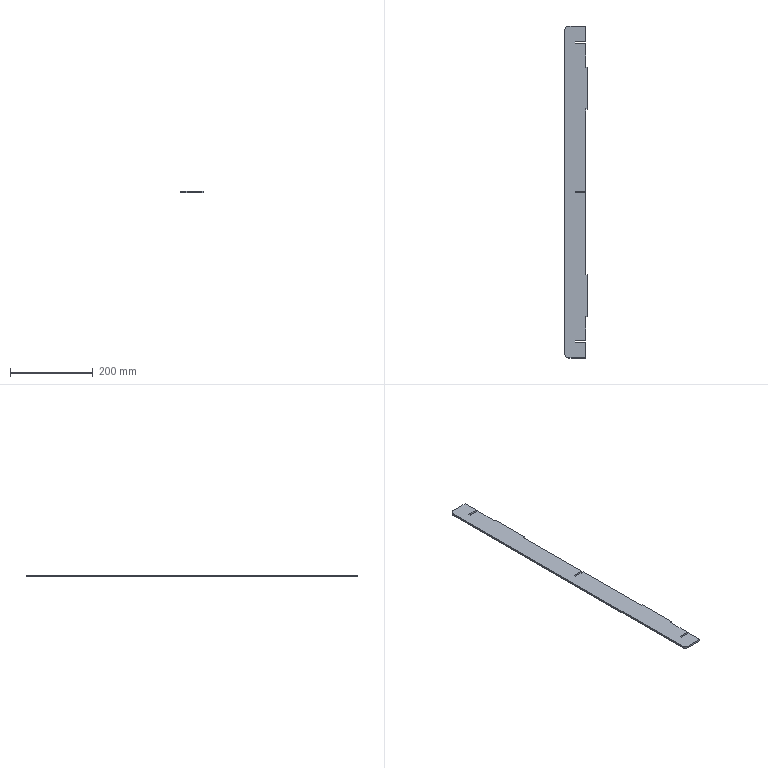Part | SolidWorks | features FlatPattern 1, SMBaseFlange 1, SheetMetal 1 | 1 solid | 28 faces | box 54 x 800 x 4.5 mm | volume 181888 mm3 | plane 26 | cylinder 2 | commonest cylinder face diameters 20 x2
STEP:
#1=CARTESIAN_POINT('',(1108.071,318.842,0.));
#2=VERTEX_POINT('',#1);
#3=CARTESIAN_POINT('',(1108.071,356.592,0.));
#4=VERTEX_POINT('',#3);
#5=CARTESIAN_POINT('',(1108.071,356.592,0.));
#6=DIRECTION('',(0.,1.,0.));
#7=VECTOR('',#6,1000.);
#8=LINE('',#5,#7);
#9=EDGE_CURVE('',#2,#4,#8,.T.);
#10=ORIENTED_EDGE('',*,*,#9,.F.);
#11=CARTESIAN_POINT('',(1108.071,318.842,-4.5));
#12=VERTEX_POINT('',#11);
#13=CARTESIAN_POINT('',(1108.071,318.842,-4.5));
#14=DIRECTION('',(0.,0.,1.));
#15=VECTOR('',#14,1000.);
#16=LINE('',#13,#15);
#17=EDGE_CURVE('',#12,#2,#16,.T.);
#18=ORIENTED_EDGE('',*,*,#17,.F.);
#19=CARTESIAN_POINT('',(1108.071,356.592,-4.5));
#20=VERTEX_POINT('',#19);
#21=CARTESIAN_POINT('',(1108.071,356.592,-4.5));
#22=DIRECTION('',(0.,1.,0.));
#23=VECTOR('',#22,1000.);
#24=LINE('',#21,#23);
#25=EDGE_CURVE('',#12,#20,#24,.T.);
#26=ORIENTED_EDGE('',*,*,#25,.T.);
#27=CARTESIAN_POINT('',(1108.071,356.592,-4.5));
#28=DIRECTION('',(0.,0.,1.));
#29=VECTOR('',#28,1000.);
#30=LINE('',#27,#29);
#31=EDGE_CURVE('',#20,#4,#30,.T.);
#32=ORIENTED_EDGE('',*,*,#31,.T.);
#33=EDGE_LOOP('',(#10,#18,#26,#32));
#34=FACE_OUTER_BOUND('',#33,.T.);
#35=CARTESIAN_POINT('',(1108.071,356.592,-4.5));
#36=DIRECTION('',(1.,0.,0.));
#37=DIRECTION('',(0.,0.,-1.));
#38=AXIS2_PLACEMENT_3D('',#35,#36,#37);
#39=PLANE('',#38);
#40=ADVANCED_FACE('',(#34),#39,.T.);
#41=CARTESIAN_POINT('',(1083.071,318.842,0.));
#42=VERTEX_POINT('',#41);
#43=CARTESIAN_POINT('',(1108.071,318.842,0.));
#44=DIRECTION('',(1.,0.,0.));
#45=VECTOR('',#44,1000.);
#46=LINE('',#43,#45);
#47=EDGE_CURVE('',#42,#2,#46,.T.);
#48=ORIENTED_EDGE('',*,*,#47,.F.);
#49=CARTESIAN_POINT('',(1083.071,318.842,-4.5));
#50=VERTEX_POINT('',#49);
#51=CARTESIAN_POINT('',(1083.071,318.842,-4.5));
#52=DIRECTION('',(0.,0.,1.));
#53=VECTOR('',#52,1000.);
#54=LINE('',#51,#53);
#55=EDGE_CURVE('',#50,#42,#54,.T.);
#56=ORIENTED_EDGE('',*,*,#55,.F.);
#57=CARTESIAN_POINT('',(1108.071,318.842,-4.5));
#58=DIRECTION('',(1.,0.,0.));
#59=VECTOR('',#58,1000.);
#60=LINE('',#57,#59);
#61=EDGE_CURVE('',#50,#12,#60,.T.);
#62=ORIENTED_EDGE('',*,*,#61,.T.);
#63=ORIENTED_EDGE('',*,*,#17,.T.);
#64=EDGE_LOOP('',(#48,#56,#62,#63));
#65=FACE_OUTER_BOUND('',#64,.T.);
#66=CARTESIAN_POINT('',(1108.071,318.842,-4.5));
#67=DIRECTION('',(0.,-1.,0.));
#68=DIRECTION('',(0.,0.,-1.));
#69=AXIS2_PLACEMENT_3D('',#66,#67,#68);
#70=PLANE('',#69);
#71=ADVANCED_FACE('',(#65),#70,.T.);
#72=CARTESIAN_POINT('',(1083.071,314.342,0.));
#73=VERTEX_POINT('',#72);
#74=CARTESIAN_POINT('',(1083.071,318.842,0.));
#75=DIRECTION('',(0.,1.,0.));
#76=VECTOR('',#75,1000.);
#77=LINE('',#74,#76);
#78=EDGE_CURVE('',#73,#42,#77,.T.);
#79=ORIENTED_EDGE('',*,*,#78,.F.);
#80=CARTESIAN_POINT('',(1083.071,314.342,-4.5));
#81=VERTEX_POINT('',#80);
#82=CARTESIAN_POINT('',(1083.071,314.342,-4.5));
#83=DIRECTION('',(0.,0.,1.));
#84=VECTOR('',#83,1000.);
#85=LINE('',#82,#84);
#86=EDGE_CURVE('',#81,#73,#85,.T.);
#87=ORIENTED_EDGE('',*,*,#86,.F.);
#88=CARTESIAN_POINT('',(1083.071,318.842,-4.5));
#89=DIRECTION('',(0.,1.,0.));
#90=VECTOR('',#89,1000.);
#91=LINE('',#88,#90);
#92=EDGE_CURVE('',#81,#50,#91,.T.);
#93=ORIENTED_EDGE('',*,*,#92,.T.);
#94=ORIENTED_EDGE('',*,*,#55,.T.);
#95=EDGE_LOOP('',(#79,#87,#93,#94));
#96=FACE_OUTER_BOUND('',#95,.T.);
#97=CARTESIAN_POINT('',(1083.071,318.842,-4.5));
#98=DIRECTION('',(1.,0.,0.));
#99=DIRECTION('',(0.,0.,-1.));
#100=AXIS2_PLACEMENT_3D('',#97,#98,#99);
#101=PLANE('',#100);
#102=ADVANCED_FACE('',(#96),#101,.T.);
#103=CARTESIAN_POINT('',(1108.071,314.342,0.));
#104=VERTEX_POINT('',#103);
#105=CARTESIAN_POINT('',(1083.071,314.342,0.));
#106=DIRECTION('',(-1.,0.,0.));
#107=VECTOR('',#106,1000.);
#108=LINE('',#105,#107);
#109=EDGE_CURVE('',#104,#73,#108,.T.);
#110=ORIENTED_EDGE('',*,*,#109,.F.);
#111=CARTESIAN_POINT('',(1108.071,314.342,-4.5));
#112=VERTEX_POINT('',#111);
#113=CARTESIAN_POINT('',(1108.071,314.342,-4.5));
#114=DIRECTION('',(0.,0.,1.));
#115=VECTOR('',#114,1000.);
#116=LINE('',#113,#115);
#117=EDGE_CURVE('',#112,#104,#116,.T.);
#118=ORIENTED_EDGE('',*,*,#117,.F.);
#119=CARTESIAN_POINT('',(1083.071,314.342,-4.5));
#120=DIRECTION('',(-1.,0.,0.));
#121=VECTOR('',#120,1000.);
#122=LINE('',#119,#121);
#123=EDGE_CURVE('',#112,#81,#122,.T.);
#124=ORIENTED_EDGE('',*,*,#123,.T.);
#125=ORIENTED_EDGE('',*,*,#86,.T.);
#126=EDGE_LOOP('',(#110,#118,#124,#125));
#127=FACE_OUTER_BOUND('',#126,.T.);
#128=CARTESIAN_POINT('',(1083.071,314.342,-4.5));
#129=DIRECTION('',(0.,1.,0.));
#130=DIRECTION('',(0.,0.,1.));
#131=AXIS2_PLACEMENT_3D('',#128,#129,#130);
#132=PLANE('',#131);
#133=ADVANCED_FACE('',(#127),#132,.T.);
#134=CARTESIAN_POINT('',(1108.071,256.592,0.));
#135=VERTEX_POINT('',#134);
#136=CARTESIAN_POINT('',(1108.071,314.342,0.));
#137=DIRECTION('',(0.,1.,0.));
#138=VECTOR('',#137,1000.);
#139=LINE('',#136,#138);
#140=EDGE_CURVE('',#135,#104,#139,.T.);
#141=ORIENTED_EDGE('',*,*,#140,.F.);
#142=CARTESIAN_POINT('',(1108.071,256.592,-4.5));
#143=VERTEX_POINT('',#142);
#144=CARTESIAN_POINT('',(1108.071,256.592,-4.5));
#145=DIRECTION('',(0.,0.,1.));
#146=VECTOR('',#145,1000.);
#147=LINE('',#144,#146);
#148=EDGE_CURVE('',#143,#135,#147,.T.);
#149=ORIENTED_EDGE('',*,*,#148,.F.);
#150=CARTESIAN_POINT('',(1108.071,314.342,-4.5));
#151=DIRECTION('',(0.,1.,0.));
#152=VECTOR('',#151,1000.);
#153=LINE('',#150,#152);
#154=EDGE_CURVE('',#143,#112,#153,.T.);
#155=ORIENTED_EDGE('',*,*,#154,.T.);
#156=ORIENTED_EDGE('',*,*,#117,.T.);
#157=EDGE_LOOP('',(#141,#149,#155,#156));
#158=FACE_OUTER_BOUND('',#157,.T.);
#159=CARTESIAN_POINT('',(1108.071,314.342,-4.5));
#160=DIRECTION('',(1.,0.,0.));
#161=DIRECTION('',(0.,0.,-1.));
#162=AXIS2_PLACEMENT_3D('',#159,#160,#161);
#163=PLANE('',#162);
#164=ADVANCED_FACE('',(#158),#163,.T.);
#165=CARTESIAN_POINT('',(1112.071,256.592,0.));
#166=VERTEX_POINT('',#165);
#167=CARTESIAN_POINT('',(1108.071,256.592,0.));
#168=DIRECTION('',(-1.,0.,0.));
#169=VECTOR('',#168,1000.);
#170=LINE('',#167,#169);
#171=EDGE_CURVE('',#166,#135,#170,.T.);
#172=ORIENTED_EDGE('',*,*,#171,.F.);
#173=CARTESIAN_POINT('',(1112.071,256.592,-4.5));
#174=VERTEX_POINT('',#173);
#175=CARTESIAN_POINT('',(1112.071,256.592,-4.5));
#176=DIRECTION('',(0.,0.,1.));
#177=VECTOR('',#176,1000.);
#178=LINE('',#175,#177);
#179=EDGE_CURVE('',#174,#166,#178,.T.);
#180=ORIENTED_EDGE('',*,*,#179,.F.);
#181=CARTESIAN_POINT('',(1108.071,256.592,-4.5));
#182=DIRECTION('',(-1.,0.,0.));
#183=VECTOR('',#182,1000.);
#184=LINE('',#181,#183);
#185=EDGE_CURVE('',#174,#143,#184,.T.);
#186=ORIENTED_EDGE('',*,*,#185,.T.);
#187=ORIENTED_EDGE('',*,*,#148,.T.);
#188=EDGE_LOOP('',(#172,#180,#186,#187));
#189=FACE_OUTER_BOUND('',#188,.T.);
#190=CARTESIAN_POINT('',(1108.071,256.592,-4.5));
#191=DIRECTION('',(0.,1.,0.));
#192=DIRECTION('',(0.,0.,1.));
#193=AXIS2_PLACEMENT_3D('',#190,#191,#192);
#194=PLANE('',#193);
#195=ADVANCED_FACE('',(#189),#194,.T.);
#196=CARTESIAN_POINT('',(1112.071,156.592,0.));
#197=VERTEX_POINT('',#196);
#198=CARTESIAN_POINT('',(1112.071,256.592,0.));
#199=DIRECTION('',(0.,1.,0.));
#200=VECTOR('',#199,1000.);
#201=LINE('',#198,#200);
#202=EDGE_CURVE('',#197,#166,#201,.T.);
#203=ORIENTED_EDGE('',*,*,#202,.F.);
#204=CARTESIAN_POINT('',(1112.071,156.592,-4.5));
#205=VERTEX_POINT('',#204);
#206=CARTESIAN_POINT('',(1112.071,156.592,-4.5));
#207=DIRECTION('',(0.,0.,1.));
#208=VECTOR('',#207,1000.);
#209=LINE('',#206,#208);
#210=EDGE_CURVE('',#205,#197,#209,.T.);
#211=ORIENTED_EDGE('',*,*,#210,.F.);
#212=CARTESIAN_POINT('',(1112.071,256.592,-4.5));
#213=DIRECTION('',(0.,1.,0.));
#214=VECTOR('',#213,1000.);
#215=LINE('',#212,#214);
#216=EDGE_CURVE('',#205,#174,#215,.T.);
#217=ORIENTED_EDGE('',*,*,#216,.T.);
#218=ORIENTED_EDGE('',*,*,#179,.T.);
#219=EDGE_LOOP('',(#203,#211,#217,#218));
#220=FACE_OUTER_BOUND('',#219,.T.);
#221=CARTESIAN_POINT('',(1112.071,256.592,-4.5));
#222=DIRECTION('',(1.,0.,0.));
#223=DIRECTION('',(0.,1.,0.));
#224=AXIS2_PLACEMENT_3D('',#221,#222,#223);
#225=PLANE('',#224);
#226=ADVANCED_FACE('',(#220),#225,.T.);
#227=CARTESIAN_POINT('',(1108.071,156.592,0.));
#228=VERTEX_POINT('',#227);
#229=CARTESIAN_POINT('',(1112.071,156.592,0.));
#230=DIRECTION('',(1.,0.,0.));
#231=VECTOR('',#230,1000.);
#232=LINE('',#229,#231);
#233=EDGE_CURVE('',#228,#197,#232,.T.);
#234=ORIENTED_EDGE('',*,*,#233,.F.);
#235=CARTESIAN_POINT('',(1108.071,156.592,-4.5));
#236=VERTEX_POINT('',#235);
#237=CARTESIAN_POINT('',(1108.071,156.592,-4.5));
#238=DIRECTION('',(0.,0.,1.));
#239=VECTOR('',#238,1000.);
#240=LINE('',#237,#239);
#241=EDGE_CURVE('',#236,#228,#240,.T.);
#242=ORIENTED_EDGE('',*,*,#241,.F.);
#243=CARTESIAN_POINT('',(1112.071,156.592,-4.5));
#244=DIRECTION('',(1.,0.,0.));
#245=VECTOR('',#244,1000.);
#246=LINE('',#243,#245);
#247=EDGE_CURVE('',#236,#205,#246,.T.);
#248=ORIENTED_EDGE('',*,*,#247,.T.);
#249=ORIENTED_EDGE('',*,*,#210,.T.);
#250=EDGE_LOOP('',(#234,#242,#248,#249));
#251=FACE_OUTER_BOUND('',#250,.T.);
#252=CARTESIAN_POINT('',(1112.071,156.592,-4.5));
#253=DIRECTION('',(0.,-1.,0.));
#254=DIRECTION('',(0.,0.,-1.));
#255=AXIS2_PLACEMENT_3D('',#252,#253,#254);
#256=PLANE('',#255);
#257=ADVANCED_FACE('',(#251),#256,.T.);
#258=CARTESIAN_POINT('',(1108.071,-41.158,0.));
#259=VERTEX_POINT('',#258);
#260=CARTESIAN_POINT('',(1108.071,156.592,0.));
#261=DIRECTION('',(0.,1.,0.));
#262=VECTOR('',#261,1000.);
#263=LINE('',#260,#262);
#264=EDGE_CURVE('',#259,#228,#263,.T.);
#265=ORIENTED_EDGE('',*,*,#264,.F.);
#266=CARTESIAN_POINT('',(1108.071,-41.158,-4.5));
#267=VERTEX_POINT('',#266);
#268=CARTESIAN_POINT('',(1108.071,-41.158,-4.5));
#269=DIRECTION('',(0.,0.,1.));
#270=VECTOR('',#269,1000.);
#271=LINE('',#268,#270);
#272=EDGE_CURVE('',#267,#259,#271,.T.);
#273=ORIENTED_EDGE('',*,*,#272,.F.);
#274=CARTESIAN_POINT('',(1108.071,156.592,-4.5));
#275=DIRECTION('',(0.,1.,0.));
#276=VECTOR('',#275,1000.);
#277=LINE('',#274,#276);
#278=EDGE_CURVE('',#267,#236,#277,.T.);
#279=ORIENTED_EDGE('',*,*,#278,.T.);
#280=ORIENTED_EDGE('',*,*,#241,.T.);
#281=EDGE_LOOP('',(#265,#273,#279,#280));
#282=FACE_OUTER_BOUND('',#281,.T.);
#283=CARTESIAN_POINT('',(1108.071,156.592,-4.5));
#284=DIRECTION('',(1.,0.,0.));
#285=DIRECTION('',(0.,0.,-1.));
#286=AXIS2_PLACEMENT_3D('',#283,#284,#285);
#287=PLANE('',#286);
#288=ADVANCED_FACE('',(#282),#287,.T.);
#289=CARTESIAN_POINT('',(1083.071,-41.158,0.));
#290=VERTEX_POINT('',#289);
#291=CARTESIAN_POINT('',(1108.071,-41.158,0.));
#292=DIRECTION('',(1.,0.,0.));
#293=VECTOR('',#292,1000.);
#294=LINE('',#291,#293);
#295=EDGE_CURVE('',#290,#259,#294,.T.);
#296=ORIENTED_EDGE('',*,*,#295,.F.);
#297=CARTESIAN_POINT('',(1083.071,-41.158,-4.5));
#298=VERTEX_POINT('',#297);
#299=CARTESIAN_POINT('',(1083.071,-41.158,-4.5));
#300=DIRECTION('',(0.,0.,1.));
#301=VECTOR('',#300,1000.);
#302=LINE('',#299,#301);
#303=EDGE_CURVE('',#298,#290,#302,.T.);
#304=ORIENTED_EDGE('',*,*,#303,.F.);
#305=CARTESIAN_POINT('',(1108.071,-41.158,-4.5));
#306=DIRECTION('',(1.,0.,0.));
#307=VECTOR('',#306,1000.);
#308=LINE('',#305,#307);
#309=EDGE_CURVE('',#298,#267,#308,.T.);
#310=ORIENTED_EDGE('',*,*,#309,.T.);
#311=ORIENTED_EDGE('',*,*,#272,.T.);
#312=EDGE_LOOP('',(#296,#304,#310,#311));
#313=FACE_OUTER_BOUND('',#312,.T.);
#314=CARTESIAN_POINT('',(1108.071,-41.158,-4.5));
#315=DIRECTION('',(0.,-1.,0.));
#316=DIRECTION('',(0.,0.,-1.));
#317=AXIS2_PLACEMENT_3D('',#314,#315,#316);
#318=PLANE('',#317);
#319=ADVANCED_FACE('',(#313),#318,.T.);
#320=CARTESIAN_POINT('',(1083.071,-45.658,0.));
#321=VERTEX_POINT('',#320);
#322=CARTESIAN_POINT('',(1083.071,-41.158,0.));
#323=DIRECTION('',(0.,1.,0.));
#324=VECTOR('',#323,1000.);
#325=LINE('',#322,#324);
#326=EDGE_CURVE('',#321,#290,#325,.T.);
#327=ORIENTED_EDGE('',*,*,#326,.F.);
#328=CARTESIAN_POINT('',(1083.071,-45.658,-4.5));
#329=VERTEX_POINT('',#328);
#330=CARTESIAN_POINT('',(1083.071,-45.658,-4.5));
#331=DIRECTION('',(0.,0.,1.));
#332=VECTOR('',#331,1000.);
#333=LINE('',#330,#332);
#334=EDGE_CURVE('',#329,#321,#333,.T.);
#335=ORIENTED_EDGE('',*,*,#334,.F.);
#336=CARTESIAN_POINT('',(1083.071,-41.158,-4.5));
#337=DIRECTION('',(0.,1.,0.));
#338=VECTOR('',#337,1000.);
#339=LINE('',#336,#338);
#340=EDGE_CURVE('',#329,#298,#339,.T.);
#341=ORIENTED_EDGE('',*,*,#340,.T.);
#342=ORIENTED_EDGE('',*,*,#303,.T.);
#343=EDGE_LOOP('',(#327,#335,#341,#342));
#344=FACE_OUTER_BOUND('',#343,.T.);
#345=CARTESIAN_POINT('',(1083.071,-41.158,-4.5));
#346=DIRECTION('',(1.,0.,0.));
#347=DIRECTION('',(0.,0.,-1.));
#348=AXIS2_PLACEMENT_3D('',#345,#346,#347);
#349=PLANE('',#348);
#350=ADVANCED_FACE('',(#344),#349,.T.);
#351=CARTESIAN_POINT('',(1108.071,-45.658,0.));
#352=VERTEX_POINT('',#351);
#353=CARTESIAN_POINT('',(1083.071,-45.658,0.));
#354=DIRECTION('',(-1.,0.,0.));
#355=VECTOR('',#354,1000.);
#356=LINE('',#353,#355);
#357=EDGE_CURVE('',#352,#321,#356,.T.);
#358=ORIENTED_EDGE('',*,*,#357,.F.);
#359=CARTESIAN_POINT('',(1108.071,-45.658,-4.5));
#360=VERTEX_POINT('',#359);
#361=CARTESIAN_POINT('',(1108.071,-45.658,-4.5));
#362=DIRECTION('',(0.,0.,1.));
#363=VECTOR('',#362,1000.);
#364=LINE('',#361,#363);
#365=EDGE_CURVE('',#360,#352,#364,.T.);
#366=ORIENTED_EDGE('',*,*,#365,.F.);
#367=CARTESIAN_POINT('',(1083.071,-45.658,-4.5));
#368=DIRECTION('',(-1.,0.,0.));
#369=VECTOR('',#368,1000.);
#370=LINE('',#367,#369);
#371=EDGE_CURVE('',#360,#329,#370,.T.);
#372=ORIENTED_EDGE('',*,*,#371,.T.);
#373=ORIENTED_EDGE('',*,*,#334,.T.);
#374=EDGE_LOOP('',(#358,#366,#372,#373));
#375=FACE_OUTER_BOUND('',#374,.T.);
#376=CARTESIAN_POINT('',(1083.071,-45.658,-4.5));
#377=DIRECTION('',(0.,1.,0.));
#378=DIRECTION('',(0.,0.,1.));
#379=AXIS2_PLACEMENT_3D('',#376,#377,#378);
#380=PLANE('',#379);
#381=ADVANCED_FACE('',(#375),#380,.T.);
#382=CARTESIAN_POINT('',(1108.071,-243.408,0.));
#383=VERTEX_POINT('',#382);
#384=CARTESIAN_POINT('',(1108.071,-45.658,0.));
#385=DIRECTION('',(0.,1.,0.));
#386=VECTOR('',#385,1000.);
#387=LINE('',#384,#386);
#388=EDGE_CURVE('',#383,#352,#387,.T.);
#389=ORIENTED_EDGE('',*,*,#388,.F.);
#390=CARTESIAN_POINT('',(1108.071,-243.408,-4.5));
#391=VERTEX_POINT('',#390);
#392=CARTESIAN_POINT('',(1108.071,-243.408,-4.5));
#393=DIRECTION('',(0.,0.,1.));
#394=VECTOR('',#393,1000.);
#395=LINE('',#392,#394);
#396=EDGE_CURVE('',#391,#383,#395,.T.);
#397=ORIENTED_EDGE('',*,*,#396,.F.);
#398=CARTESIAN_POINT('',(1108.071,-45.658,-4.5));
#399=DIRECTION('',(0.,1.,0.));
#400=VECTOR('',#399,1000.);
#401=LINE('',#398,#400);
#402=EDGE_CURVE('',#391,#360,#401,.T.);
#403=ORIENTED_EDGE('',*,*,#402,.T.);
#404=ORIENTED_EDGE('',*,*,#365,.T.);
#405=EDGE_LOOP('',(#389,#397,#403,#404));
#406=FACE_OUTER_BOUND('',#405,.T.);
#407=CARTESIAN_POINT('',(1108.071,-45.658,-4.5));
#408=DIRECTION('',(1.,0.,0.));
#409=DIRECTION('',(0.,0.,-1.));
#410=AXIS2_PLACEMENT_3D('',#407,#408,#409);
#411=PLANE('',#410);
#412=ADVANCED_FACE('',(#406),#411,.T.);
#413=CARTESIAN_POINT('',(1112.071,-243.408,0.));
#414=VERTEX_POINT('',#413);
#415=CARTESIAN_POINT('',(1112.071,-243.408,0.));
#416=DIRECTION('',(-1.,0.,0.));
#417=VECTOR('',#416,1000.);
#418=LINE('',#415,#417);
#419=EDGE_CURVE('',#414,#383,#418,.T.);
#420=ORIENTED_EDGE('',*,*,#419,.F.);
#421=CARTESIAN_POINT('',(1112.071,-243.408,-4.5));
#422=VERTEX_POINT('',#421);
#423=CARTESIAN_POINT('',(1112.071,-243.408,-4.5));
#424=DIRECTION('',(0.,0.,1.));
#425=VECTOR('',#424,1000.);
#426=LINE('',#423,#425);
#427=EDGE_CURVE('',#422,#414,#426,.T.);
#428=ORIENTED_EDGE('',*,*,#427,.F.);
#429=CARTESIAN_POINT('',(1112.071,-243.408,-4.5));
#430=DIRECTION('',(-1.,0.,0.));
#431=VECTOR('',#430,1000.);
#432=LINE('',#429,#431);
#433=EDGE_CURVE('',#422,#391,#432,.T.);
#434=ORIENTED_EDGE('',*,*,#433,.T.);
#435=ORIENTED_EDGE('',*,*,#396,.T.);
#436=EDGE_LOOP('',(#420,#428,#434,#435));
#437=FACE_OUTER_BOUND('',#436,.T.);
#438=CARTESIAN_POINT('',(1112.071,-243.408,-4.5));
#439=DIRECTION('',(0.,1.,0.));
#440=DIRECTION('',(-1.,0.,0.));
#441=AXIS2_PLACEMENT_3D('',#438,#439,#440);
#442=PLANE('',#441);
#443=ADVANCED_FACE('',(#437),#442,.T.);
#444=CARTESIAN_POINT('',(1112.071,-343.408,0.));
#445=VERTEX_POINT('',#444);
#446=CARTESIAN_POINT('',(1112.071,-343.408,0.));
#447=DIRECTION('',(0.,1.,0.));
#448=VECTOR('',#447,1000.);
#449=LINE('',#446,#448);
#450=EDGE_CURVE('',#445,#414,#449,.T.);
#451=ORIENTED_EDGE('',*,*,#450,.F.);
#452=CARTESIAN_POINT('',(1112.071,-343.408,-4.5));
#453=VERTEX_POINT('',#452);
#454=CARTESIAN_POINT('',(1112.071,-343.408,-4.5));
#455=DIRECTION('',(0.,0.,1.));
#456=VECTOR('',#455,1000.);
#457=LINE('',#454,#456);
#458=EDGE_CURVE('',#453,#445,#457,.T.);
#459=ORIENTED_EDGE('',*,*,#458,.F.);
#460=CARTESIAN_POINT('',(1112.071,-343.408,-4.5));
#461=DIRECTION('',(0.,1.,0.));
#462=VECTOR('',#461,1000.);
#463=LINE('',#460,#462);
#464=EDGE_CURVE('',#453,#422,#463,.T.);
#465=ORIENTED_EDGE('',*,*,#464,.T.);
#466=ORIENTED_EDGE('',*,*,#427,.T.);
#467=EDGE_LOOP('',(#451,#459,#465,#466));
#468=FACE_OUTER_BOUND('',#467,.T.);
#469=CARTESIAN_POINT('',(1112.071,-343.408,-4.5));
#470=DIRECTION('',(1.,0.,0.));
#471=DIRECTION('',(0.,0.,-1.));
#472=AXIS2_PLACEMENT_3D('',#469,#470,#471);
#473=PLANE('',#472);
#474=ADVANCED_FACE('',(#468),#473,.T.);
#475=CARTESIAN_POINT('',(1108.071,-343.408,0.));
#476=VERTEX_POINT('',#475);
#477=CARTESIAN_POINT('',(1108.071,-343.408,0.));
#478=DIRECTION('',(1.,0.,0.));
#479=VECTOR('',#478,1000.);
#480=LINE('',#477,#479);
#481=EDGE_CURVE('',#476,#445,#480,.T.);
#482=ORIENTED_EDGE('',*,*,#481,.F.);
#483=CARTESIAN_POINT('',(1108.071,-343.408,-4.5));
#484=VERTEX_POINT('',#483);
#485=CARTESIAN_POINT('',(1108.071,-343.408,-4.5));
#486=DIRECTION('',(0.,0.,1.));
#487=VECTOR('',#486,1000.);
#488=LINE('',#485,#487);
#489=EDGE_CURVE('',#484,#476,#488,.T.);
#490=ORIENTED_EDGE('',*,*,#489,.F.);
#491=CARTESIAN_POINT('',(1108.071,-343.408,-4.5));
#492=DIRECTION('',(1.,0.,0.));
#493=VECTOR('',#492,1000.);
#494=LINE('',#491,#493);
#495=EDGE_CURVE('',#484,#453,#494,.T.);
#496=ORIENTED_EDGE('',*,*,#495,.T.);
#497=ORIENTED_EDGE('',*,*,#458,.T.);
#498=EDGE_LOOP('',(#482,#490,#496,#497));
#499=FACE_OUTER_BOUND('',#498,.T.);
#500=CARTESIAN_POINT('',(1108.071,-343.408,-4.5));
#501=DIRECTION('',(0.,-1.,0.));
#502=DIRECTION('',(0.,0.,-1.));
#503=AXIS2_PLACEMENT_3D('',#500,#501,#502);
#504=PLANE('',#503);
#505=ADVANCED_FACE('',(#499),#504,.T.);
#506=CARTESIAN_POINT('',(1108.071,-401.158,0.));
#507=VERTEX_POINT('',#506);
#508=CARTESIAN_POINT('',(1108.071,-343.408,0.));
#509=DIRECTION('',(0.,1.,0.));
#510=VECTOR('',#509,1000.);
#511=LINE('',#508,#510);
#512=EDGE_CURVE('',#507,#476,#511,.T.);
#513=ORIENTED_EDGE('',*,*,#512,.F.);
#514=CARTESIAN_POINT('',(1108.071,-401.158,-4.5));
#515=VERTEX_POINT('',#514);
#516=CARTESIAN_POINT('',(1108.071,-401.158,-4.5));
#517=DIRECTION('',(0.,0.,1.));
#518=VECTOR('',#517,1000.);
#519=LINE('',#516,#518);
#520=EDGE_CURVE('',#515,#507,#519,.T.);
#521=ORIENTED_EDGE('',*,*,#520,.F.);
#522=CARTESIAN_POINT('',(1108.071,-343.408,-4.5));
#523=DIRECTION('',(0.,1.,0.));
#524=VECTOR('',#523,1000.);
#525=LINE('',#522,#524);
#526=EDGE_CURVE('',#515,#484,#525,.T.);
#527=ORIENTED_EDGE('',*,*,#526,.T.);
#528=ORIENTED_EDGE('',*,*,#489,.T.);
#529=EDGE_LOOP('',(#513,#521,#527,#528));
#530=FACE_OUTER_BOUND('',#529,.T.);
#531=CARTESIAN_POINT('',(1108.071,-343.408,-4.5));
#532=DIRECTION('',(1.,0.,0.));
#533=DIRECTION('',(0.,0.,-1.));
#534=AXIS2_PLACEMENT_3D('',#531,#532,#533);
#535=PLANE('',#534);
#536=ADVANCED_FACE('',(#530),#535,.T.);
#537=CARTESIAN_POINT('',(1083.071,-401.158,0.));
#538=VERTEX_POINT('',#537);
#539=CARTESIAN_POINT('',(1108.071,-401.158,0.));
#540=DIRECTION('',(1.,0.,0.));
#541=VECTOR('',#540,1000.);
#542=LINE('',#539,#541);
#543=EDGE_CURVE('',#538,#507,#542,.T.);
#544=ORIENTED_EDGE('',*,*,#543,.F.);
#545=CARTESIAN_POINT('',(1083.071,-401.158,-4.5));
#546=VERTEX_POINT('',#545);
#547=CARTESIAN_POINT('',(1083.071,-401.158,-4.5));
#548=DIRECTION('',(0.,0.,1.));
#549=VECTOR('',#548,1000.);
#550=LINE('',#547,#549);
#551=EDGE_CURVE('',#546,#538,#550,.T.);
#552=ORIENTED_EDGE('',*,*,#551,.F.);
#553=CARTESIAN_POINT('',(1108.071,-401.158,-4.5));
#554=DIRECTION('',(1.,0.,0.));
#555=VECTOR('',#554,1000.);
#556=LINE('',#553,#555);
#557=EDGE_CURVE('',#546,#515,#556,.T.);
#558=ORIENTED_EDGE('',*,*,#557,.T.);
#559=ORIENTED_EDGE('',*,*,#520,.T.);
#560=EDGE_LOOP('',(#544,#552,#558,#559));
#561=FACE_OUTER_BOUND('',#560,.T.);
#562=CARTESIAN_POINT('',(1108.071,-401.158,-4.5));
#563=DIRECTION('',(0.,-1.,0.));
#564=DIRECTION('',(0.,0.,-1.));
#565=AXIS2_PLACEMENT_3D('',#562,#563,#564);
#566=PLANE('',#565);
#567=ADVANCED_FACE('',(#561),#566,.T.);
#568=CARTESIAN_POINT('',(1083.071,-405.658,0.));
#569=VERTEX_POINT('',#568);
#570=CARTESIAN_POINT('',(1083.071,-401.158,0.));
#571=DIRECTION('',(0.,1.,0.));
#572=VECTOR('',#571,1000.);
#573=LINE('',#570,#572);
#574=EDGE_CURVE('',#569,#538,#573,.T.);
#575=ORIENTED_EDGE('',*,*,#574,.F.);
#576=CARTESIAN_POINT('',(1083.071,-405.658,-4.5));
#577=VERTEX_POINT('',#576);
#578=CARTESIAN_POINT('',(1083.071,-405.658,-4.5));
#579=DIRECTION('',(0.,0.,1.));
#580=VECTOR('',#579,1000.);
#581=LINE('',#578,#580);
#582=EDGE_CURVE('',#577,#569,#581,.T.);
#583=ORIENTED_EDGE('',*,*,#582,.F.);
#584=CARTESIAN_POINT('',(1083.071,-401.158,-4.5));
#585=DIRECTION('',(0.,1.,0.));
#586=VECTOR('',#585,1000.);
#587=LINE('',#584,#586);
#588=EDGE_CURVE('',#577,#546,#587,.T.);
#589=ORIENTED_EDGE('',*,*,#588,.T.);
#590=ORIENTED_EDGE('',*,*,#551,.T.);
#591=EDGE_LOOP('',(#575,#583,#589,#590));
#592=FACE_OUTER_BOUND('',#591,.T.);
#593=CARTESIAN_POINT('',(1083.071,-401.158,-4.5));
#594=DIRECTION('',(1.,0.,0.));
#595=DIRECTION('',(0.,0.,-1.));
#596=AXIS2_PLACEMENT_3D('',#593,#594,#595);
#597=PLANE('',#596);
#598=ADVANCED_FACE('',(#592),#597,.T.);
#599=CARTESIAN_POINT('',(1108.071,-405.658,0.));
#600=VERTEX_POINT('',#599);
#601=CARTESIAN_POINT('',(1083.071,-405.658,0.));
#602=DIRECTION('',(-1.,0.,0.));
#603=VECTOR('',#602,1000.);
#604=LINE('',#601,#603);
#605=EDGE_CURVE('',#600,#569,#604,.T.);
#606=ORIENTED_EDGE('',*,*,#605,.F.);
#607=CARTESIAN_POINT('',(1108.071,-405.658,-4.5));
#608=VERTEX_POINT('',#607);
#609=CARTESIAN_POINT('',(1108.071,-405.658,-4.5));
#610=DIRECTION('',(0.,0.,1.));
#611=VECTOR('',#610,1000.);
#612=LINE('',#609,#611);
#613=EDGE_CURVE('',#608,#600,#612,.T.);
#614=ORIENTED_EDGE('',*,*,#613,.F.);
#615=CARTESIAN_POINT('',(1083.071,-405.658,-4.5));
#616=DIRECTION('',(-1.,0.,0.));
#617=VECTOR('',#616,1000.);
#618=LINE('',#615,#617);
#619=EDGE_CURVE('',#608,#577,#618,.T.);
#620=ORIENTED_EDGE('',*,*,#619,.T.);
#621=ORIENTED_EDGE('',*,*,#582,.T.);
#622=EDGE_LOOP('',(#606,#614,#620,#621));
#623=FACE_OUTER_BOUND('',#622,.T.);
#624=CARTESIAN_POINT('',(1083.071,-405.658,-4.5));
#625=DIRECTION('',(0.,1.,0.));
#626=DIRECTION('',(0.,0.,1.));
#627=AXIS2_PLACEMENT_3D('',#624,#625,#626);
#628=PLANE('',#627);
#629=ADVANCED_FACE('',(#623),#628,.T.);
#630=CARTESIAN_POINT('',(1108.071,-443.408,0.));
#631=VERTEX_POINT('',#630);
#632=CARTESIAN_POINT('',(1108.071,-405.658,0.));
#633=DIRECTION('',(0.,1.,0.));
#634=VECTOR('',#633,1000.);
#635=LINE('',#632,#634);
#636=EDGE_CURVE('',#631,#600,#635,.T.);
#637=ORIENTED_EDGE('',*,*,#636,.F.);
#638=CARTESIAN_POINT('',(1108.071,-443.408,-4.5));
#639=VERTEX_POINT('',#638);
#640=CARTESIAN_POINT('',(1108.071,-443.408,-4.5));
#641=DIRECTION('',(0.,0.,1.));
#642=VECTOR('',#641,1000.);
#643=LINE('',#640,#642);
#644=EDGE_CURVE('',#639,#631,#643,.T.);
#645=ORIENTED_EDGE('',*,*,#644,.F.);
#646=CARTESIAN_POINT('',(1108.071,-405.658,-4.5));
#647=DIRECTION('',(0.,1.,0.));
#648=VECTOR('',#647,1000.);
#649=LINE('',#646,#648);
#650=EDGE_CURVE('',#639,#608,#649,.T.);
#651=ORIENTED_EDGE('',*,*,#650,.T.);
#652=ORIENTED_EDGE('',*,*,#613,.T.);
#653=EDGE_LOOP('',(#637,#645,#651,#652));
#654=FACE_OUTER_BOUND('',#653,.T.);
#655=CARTESIAN_POINT('',(1108.071,-405.658,-4.5));
#656=DIRECTION('',(1.,0.,0.));
#657=DIRECTION('',(0.,0.,-1.));
#658=AXIS2_PLACEMENT_3D('',#655,#656,#657);
#659=PLANE('',#658);
#660=ADVANCED_FACE('',(#654),#659,.T.);
#661=CARTESIAN_POINT('',(1068.071,-443.408,0.));
#662=VERTEX_POINT('',#661);
#663=CARTESIAN_POINT('',(1108.071,-443.408,0.));
#664=DIRECTION('',(1.,0.,0.));
#665=VECTOR('',#664,1000.);
#666=LINE('',#663,#665);
#667=EDGE_CURVE('',#662,#631,#666,.T.);
#668=ORIENTED_EDGE('',*,*,#667,.F.);
#669=CARTESIAN_POINT('',(1068.071,-443.408,-4.5));
#670=VERTEX_POINT('',#669);
#671=CARTESIAN_POINT('',(1068.071,-443.408,-4.5));
#672=DIRECTION('',(0.,0.,1.));
#673=VECTOR('',#672,1000.);
#674=LINE('',#671,#673);
#675=EDGE_CURVE('',#670,#662,#674,.T.);
#676=ORIENTED_EDGE('',*,*,#675,.F.);
#677=CARTESIAN_POINT('',(1108.071,-443.408,-4.5));
#678=DIRECTION('',(1.,0.,0.));
#679=VECTOR('',#678,1000.);
#680=LINE('',#677,#679);
#681=EDGE_CURVE('',#670,#639,#680,.T.);
#682=ORIENTED_EDGE('',*,*,#681,.T.);
#683=ORIENTED_EDGE('',*,*,#644,.T.);
#684=EDGE_LOOP('',(#668,#676,#682,#683));
#685=FACE_OUTER_BOUND('',#684,.T.);
#686=CARTESIAN_POINT('',(1108.071,-443.408,-4.5));
#687=DIRECTION('',(0.,-1.,0.));
#688=DIRECTION('',(1.,0.,0.));
#689=AXIS2_PLACEMENT_3D('',#686,#687,#688);
#690=PLANE('',#689);
#691=ADVANCED_FACE('',(#685),#690,.T.);
#692=CARTESIAN_POINT('',(1058.071,-433.408,0.));
#693=VERTEX_POINT('',#692);
#694=CARTESIAN_POINT('',(1068.071,-433.408,0.));
#695=DIRECTION('',(0.,0.,1.));
#696=DIRECTION('',(-1.,0.,0.));
#697=AXIS2_PLACEMENT_3D('',#694,#695,#696);
#698=CIRCLE('',#697,10.);
#699=EDGE_CURVE('',#693,#662,#698,.T.);
#700=ORIENTED_EDGE('',*,*,#699,.F.);
#701=CARTESIAN_POINT('',(1058.071,-433.408,-4.5));
#702=VERTEX_POINT('',#701);
#703=CARTESIAN_POINT('',(1058.071,-433.408,-4.5));
#704=DIRECTION('',(0.,0.,1.));
#705=VECTOR('',#704,1000.);
#706=LINE('',#703,#705);
#707=EDGE_CURVE('',#702,#693,#706,.T.);
#708=ORIENTED_EDGE('',*,*,#707,.F.);
#709=CARTESIAN_POINT('',(1068.071,-433.408,-4.5));
#710=DIRECTION('',(0.,0.,1.));
#711=DIRECTION('',(-1.,0.,0.));
#712=AXIS2_PLACEMENT_3D('',#709,#710,#711);
#713=CIRCLE('',#712,10.);
#714=EDGE_CURVE('',#702,#670,#713,.T.);
#715=ORIENTED_EDGE('',*,*,#714,.T.);
#716=ORIENTED_EDGE('',*,*,#675,.T.);
#717=EDGE_LOOP('',(#700,#708,#715,#716));
#718=FACE_OUTER_BOUND('',#717,.T.);
#719=CARTESIAN_POINT('',(1068.071,-433.408,-4.5));
#720=DIRECTION('',(0.,0.,1.));
#721=DIRECTION('',(1.,0.,0.));
#722=AXIS2_PLACEMENT_3D('',#719,#720,#721);
#723=CYLINDRICAL_SURFACE('',#722,10.);
#724=ADVANCED_FACE('',(#718),#723,.T.);
#725=CARTESIAN_POINT('',(1058.071,346.592,0.));
#726=VERTEX_POINT('',#725);
#727=CARTESIAN_POINT('',(1058.071,346.592,0.));
#728=DIRECTION('',(0.,-1.,0.));
#729=VECTOR('',#728,1000.);
#730=LINE('',#727,#729);
#731=EDGE_CURVE('',#726,#693,#730,.T.);
#732=ORIENTED_EDGE('',*,*,#731,.F.);
#733=CARTESIAN_POINT('',(1058.071,346.592,-4.5));
#734=VERTEX_POINT('',#733);
#735=CARTESIAN_POINT('',(1058.071,346.592,-4.5));
#736=DIRECTION('',(0.,0.,1.));
#737=VECTOR('',#736,1000.);
#738=LINE('',#735,#737);
#739=EDGE_CURVE('',#734,#726,#738,.T.);
#740=ORIENTED_EDGE('',*,*,#739,.F.);
#741=CARTESIAN_POINT('',(1058.071,346.592,-4.5));
#742=DIRECTION('',(0.,-1.,0.));
#743=VECTOR('',#742,1000.);
#744=LINE('',#741,#743);
#745=EDGE_CURVE('',#734,#702,#744,.T.);
#746=ORIENTED_EDGE('',*,*,#745,.T.);
#747=ORIENTED_EDGE('',*,*,#707,.T.);
#748=EDGE_LOOP('',(#732,#740,#746,#747));
#749=FACE_OUTER_BOUND('',#748,.T.);
#750=CARTESIAN_POINT('',(1058.071,346.592,-4.5));
#751=DIRECTION('',(-1.,0.,0.));
#752=DIRECTION('',(0.,0.,1.));
#753=AXIS2_PLACEMENT_3D('',#750,#751,#752);
#754=PLANE('',#753);
#755=ADVANCED_FACE('',(#749),#754,.T.);
#756=CARTESIAN_POINT('',(1068.071,356.592,0.));
#757=VERTEX_POINT('',#756);
#758=CARTESIAN_POINT('',(1068.071,346.592,0.));
#759=DIRECTION('',(0.,0.,1.));
#760=DIRECTION('',(1.,0.,0.));
#761=AXIS2_PLACEMENT_3D('',#758,#759,#760);
#762=CIRCLE('',#761,10.);
#763=EDGE_CURVE('',#757,#726,#762,.T.);
#764=ORIENTED_EDGE('',*,*,#763,.F.);
#765=CARTESIAN_POINT('',(1068.071,356.592,-4.5));
#766=VERTEX_POINT('',#765);
#767=CARTESIAN_POINT('',(1068.071,356.592,-4.5));
#768=DIRECTION('',(0.,0.,1.));
#769=VECTOR('',#768,1000.);
#770=LINE('',#767,#769);
#771=EDGE_CURVE('',#766,#757,#770,.T.);
#772=ORIENTED_EDGE('',*,*,#771,.F.);
#773=CARTESIAN_POINT('',(1068.071,346.592,-4.5));
#774=DIRECTION('',(0.,0.,1.));
#775=DIRECTION('',(1.,0.,0.));
#776=AXIS2_PLACEMENT_3D('',#773,#774,#775);
#777=CIRCLE('',#776,10.);
#778=EDGE_CURVE('',#766,#734,#777,.T.);
#779=ORIENTED_EDGE('',*,*,#778,.T.);
#780=ORIENTED_EDGE('',*,*,#739,.T.);
#781=EDGE_LOOP('',(#764,#772,#779,#780));
#782=FACE_OUTER_BOUND('',#781,.T.);
#783=CARTESIAN_POINT('',(1068.071,346.592,-4.5));
#784=DIRECTION('',(0.,0.,1.));
#785=DIRECTION('',(1.,0.,0.));
#786=AXIS2_PLACEMENT_3D('',#783,#784,#785);
#787=CYLINDRICAL_SURFACE('',#786,10.);
#788=ADVANCED_FACE('',(#782),#787,.T.);
#789=CARTESIAN_POINT('',(1108.071,356.592,0.));
#790=DIRECTION('',(-1.,0.,0.));
#791=VECTOR('',#790,1000.);
#792=LINE('',#789,#791);
#793=EDGE_CURVE('',#4,#757,#792,.T.);
#794=ORIENTED_EDGE('',*,*,#793,.F.);
#795=ORIENTED_EDGE('',*,*,#31,.F.);
#796=CARTESIAN_POINT('',(1108.071,356.592,-4.5));
#797=DIRECTION('',(-1.,0.,0.));
#798=VECTOR('',#797,1000.);
#799=LINE('',#796,#798);
#800=EDGE_CURVE('',#20,#766,#799,.T.);
#801=ORIENTED_EDGE('',*,*,#800,.T.);
#802=ORIENTED_EDGE('',*,*,#771,.T.);
#803=EDGE_LOOP('',(#794,#795,#801,#802));
#804=FACE_OUTER_BOUND('',#803,.T.);
#805=CARTESIAN_POINT('',(1108.071,356.592,-4.5));
#806=DIRECTION('',(0.,1.,0.));
#807=DIRECTION('',(-1.,0.,0.));
#808=AXIS2_PLACEMENT_3D('',#805,#806,#807);
#809=PLANE('',#808);
#810=ADVANCED_FACE('',(#804),#809,.T.);
#811=ORIENTED_EDGE('',*,*,#25,.F.);
#812=ORIENTED_EDGE('',*,*,#61,.F.);
#813=ORIENTED_EDGE('',*,*,#92,.F.);
#814=ORIENTED_EDGE('',*,*,#123,.F.);
#815=ORIENTED_EDGE('',*,*,#154,.F.);
#816=ORIENTED_EDGE('',*,*,#185,.F.);
#817=ORIENTED_EDGE('',*,*,#216,.F.);
#818=ORIENTED_EDGE('',*,*,#247,.F.);
#819=ORIENTED_EDGE('',*,*,#278,.F.);
#820=ORIENTED_EDGE('',*,*,#309,.F.);
#821=ORIENTED_EDGE('',*,*,#340,.F.);
#822=ORIENTED_EDGE('',*,*,#371,.F.);
#823=ORIENTED_EDGE('',*,*,#402,.F.);
#824=ORIENTED_EDGE('',*,*,#433,.F.);
#825=ORIENTED_EDGE('',*,*,#464,.F.);
#826=ORIENTED_EDGE('',*,*,#495,.F.);
#827=ORIENTED_EDGE('',*,*,#526,.F.);
#828=ORIENTED_EDGE('',*,*,#557,.F.);
#829=ORIENTED_EDGE('',*,*,#588,.F.);
#830=ORIENTED_EDGE('',*,*,#619,.F.);
#831=ORIENTED_EDGE('',*,*,#650,.F.);
#832=ORIENTED_EDGE('',*,*,#681,.F.);
#833=ORIENTED_EDGE('',*,*,#714,.F.);
#834=ORIENTED_EDGE('',*,*,#745,.F.);
#835=ORIENTED_EDGE('',*,*,#778,.F.);
#836=ORIENTED_EDGE('',*,*,#800,.F.);
#837=EDGE_LOOP('',(#811,#812,#813,#814,#815,#816,#817,#818,#819,#820,#821,#822,#823,#824,#825,#826,#827,#828,#829,#830,#831,#832,#833,#834,#835,#836));
#838=FACE_OUTER_BOUND('',#837,.T.);
#839=CARTESIAN_POINT('',(1068.071,-433.408,-4.5));
#840=DIRECTION('',(0.,0.,-1.));
#841=DIRECTION('',(-1.,0.,0.));
#842=AXIS2_PLACEMENT_3D('',#839,#840,#841);
#843=PLANE('',#842);
#844=ADVANCED_FACE('',(#838),#843,.T.);
#845=ORIENTED_EDGE('',*,*,#9,.T.);
#846=ORIENTED_EDGE('',*,*,#793,.T.);
#847=ORIENTED_EDGE('',*,*,#763,.T.);
#848=ORIENTED_EDGE('',*,*,#731,.T.);
#849=ORIENTED_EDGE('',*,*,#699,.T.);
#850=ORIENTED_EDGE('',*,*,#667,.T.);
#851=ORIENTED_EDGE('',*,*,#636,.T.);
#852=ORIENTED_EDGE('',*,*,#605,.T.);
#853=ORIENTED_EDGE('',*,*,#574,.T.);
#854=ORIENTED_EDGE('',*,*,#543,.T.);
#855=ORIENTED_EDGE('',*,*,#512,.T.);
#856=ORIENTED_EDGE('',*,*,#481,.T.);
#857=ORIENTED_EDGE('',*,*,#450,.T.);
#858=ORIENTED_EDGE('',*,*,#419,.T.);
#859=ORIENTED_EDGE('',*,*,#388,.T.);
#860=ORIENTED_EDGE('',*,*,#357,.T.);
#861=ORIENTED_EDGE('',*,*,#326,.T.);
#862=ORIENTED_EDGE('',*,*,#295,.T.);
#863=ORIENTED_EDGE('',*,*,#264,.T.);
#864=ORIENTED_EDGE('',*,*,#233,.T.);
#865=ORIENTED_EDGE('',*,*,#202,.T.);
#866=ORIENTED_EDGE('',*,*,#171,.T.);
#867=ORIENTED_EDGE('',*,*,#140,.T.);
#868=ORIENTED_EDGE('',*,*,#109,.T.);
#869=ORIENTED_EDGE('',*,*,#78,.T.);
#870=ORIENTED_EDGE('',*,*,#47,.T.);
#871=EDGE_LOOP('',(#845,#846,#847,#848,#849,#850,#851,#852,#853,#854,#855,#856,#857,#858,#859,#860,#861,#862,#863,#864,#865,#866,#867,#868,#869,#870));
#872=FACE_OUTER_BOUND('',#871,.T.);
#873=CARTESIAN_POINT('',(1068.071,-433.408,0.));
#874=DIRECTION('',(0.,0.,-1.));
#875=DIRECTION('',(-1.,0.,0.));
#876=AXIS2_PLACEMENT_3D('',#873,#874,#875);
#877=PLANE('',#876);
#878=ADVANCED_FACE('',(#872),#877,.F.);
#879=CLOSED_SHELL('',(#40,#71,#102,#133,#164,#195,#226,#257,#288,#319,#350,#381,#412,#443,#474,#505,#536,#567,#598,#629,#660,#691,#724,#755,#788,#810,#844,#878));
#880=MANIFOLD_SOLID_BREP('',#879);
#881=CARTESIAN_POINT('',(0.,0.,0.));
#882=DIRECTION('',(0.,0.,1.));
#883=DIRECTION('',(1.,0.,0.));
#884=AXIS2_PLACEMENT_3D('',#881,#882,#883);
#885=(LENGTH_UNIT()NAMED_UNIT(*)SI_UNIT(.MILLI.,.METRE.));
#886=UNCERTAINTY_MEASURE_WITH_UNIT(LENGTH_MEASURE(0.00001),#885,'','');
#887=(NAMED_UNIT(*)PLANE_ANGLE_UNIT()SI_UNIT($,.RADIAN.));
#888=(NAMED_UNIT(*)SI_UNIT($,.STERADIAN.)SOLID_ANGLE_UNIT());
#889=(GEOMETRIC_REPRESENTATION_CONTEXT(3)GLOBAL_UNCERTAINTY_ASSIGNED_CONTEXT((#886))GLOBAL_UNIT_ASSIGNED_CONTEXT((#885,#887,#888))REPRESENTATION_CONTEXT('',''));
#890=ADVANCED_BREP_SHAPE_REPRESENTATION('',(#880,#884),#889);